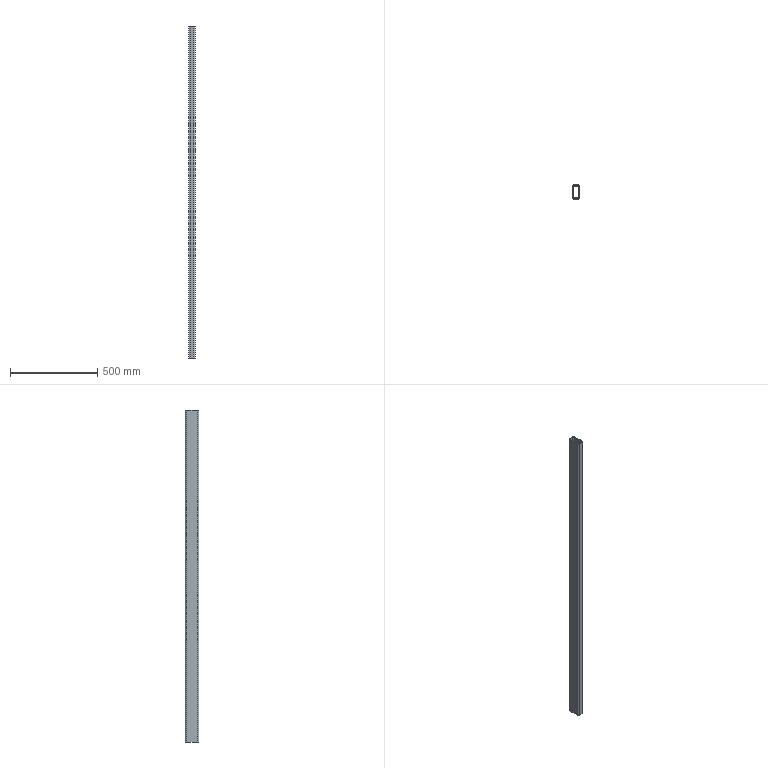Part | SolidWorks | features Extrusion 1 | 1 solid | 18 faces | box 40 x 80 x 1900 mm | volume 1967677 mm3 | plane 10 | cylinder 8 | commonest cylinder face diameters 10 x4 20 x4
STEP:
#1=CARTESIAN_POINT('',(-20.,-30.,1900.));
#2=VERTEX_POINT('',#1);
#3=CARTESIAN_POINT('',(-10.,-40.,1900.));
#4=VERTEX_POINT('',#3);
#5=CARTESIAN_POINT('',(-10.,-30.,1900.));
#6=DIRECTION('',(0.,0.,1.));
#7=DIRECTION('',(1.,0.,0.));
#8=AXIS2_PLACEMENT_3D('',#5,#6,#7);
#9=CIRCLE('',#8,10.);
#10=EDGE_CURVE('',#2,#4,#9,.T.);
#11=ORIENTED_EDGE('',*,*,#10,.T.);
#12=CARTESIAN_POINT('',(10.,-40.,1900.));
#13=VERTEX_POINT('',#12);
#14=CARTESIAN_POINT('',(-10.,-40.,1900.));
#15=DIRECTION('',(1.,0.,0.));
#16=VECTOR('',#15,1000.);
#17=LINE('',#14,#16);
#18=EDGE_CURVE('',#4,#13,#17,.T.);
#19=ORIENTED_EDGE('',*,*,#18,.T.);
#20=CARTESIAN_POINT('',(20.,-30.,1900.));
#21=VERTEX_POINT('',#20);
#22=CARTESIAN_POINT('',(10.,-30.,1900.));
#23=DIRECTION('',(0.,0.,1.));
#24=DIRECTION('',(1.,0.,0.));
#25=AXIS2_PLACEMENT_3D('',#22,#23,#24);
#26=CIRCLE('',#25,10.);
#27=EDGE_CURVE('',#13,#21,#26,.T.);
#28=ORIENTED_EDGE('',*,*,#27,.T.);
#29=CARTESIAN_POINT('',(20.,30.,1900.));
#30=VERTEX_POINT('',#29);
#31=CARTESIAN_POINT('',(20.,30.,1900.));
#32=DIRECTION('',(0.,-1.,0.));
#33=VECTOR('',#32,1000.);
#34=LINE('',#31,#33);
#35=EDGE_CURVE('',#30,#21,#34,.T.);
#36=ORIENTED_EDGE('',*,*,#35,.F.);
#37=CARTESIAN_POINT('',(10.,40.,1900.));
#38=VERTEX_POINT('',#37);
#39=CARTESIAN_POINT('',(10.,30.,1900.));
#40=DIRECTION('',(0.,0.,1.));
#41=DIRECTION('',(1.,0.,0.));
#42=AXIS2_PLACEMENT_3D('',#39,#40,#41);
#43=CIRCLE('',#42,10.);
#44=EDGE_CURVE('',#30,#38,#43,.T.);
#45=ORIENTED_EDGE('',*,*,#44,.T.);
#46=CARTESIAN_POINT('',(-10.,40.,1900.));
#47=VERTEX_POINT('',#46);
#48=CARTESIAN_POINT('',(10.,40.,1900.));
#49=DIRECTION('',(-1.,0.,0.));
#50=VECTOR('',#49,1000.);
#51=LINE('',#48,#50);
#52=EDGE_CURVE('',#38,#47,#51,.T.);
#53=ORIENTED_EDGE('',*,*,#52,.T.);
#54=CARTESIAN_POINT('',(-20.,30.,1900.));
#55=VERTEX_POINT('',#54);
#56=CARTESIAN_POINT('',(-10.,30.,1900.));
#57=DIRECTION('',(0.,0.,1.));
#58=DIRECTION('',(1.,0.,0.));
#59=AXIS2_PLACEMENT_3D('',#56,#57,#58);
#60=CIRCLE('',#59,10.);
#61=EDGE_CURVE('',#47,#55,#60,.T.);
#62=ORIENTED_EDGE('',*,*,#61,.T.);
#63=CARTESIAN_POINT('',(-20.,-30.,1900.));
#64=DIRECTION('',(0.,1.,0.));
#65=VECTOR('',#64,1000.);
#66=LINE('',#63,#65);
#67=EDGE_CURVE('',#2,#55,#66,.T.);
#68=ORIENTED_EDGE('',*,*,#67,.F.);
#69=EDGE_LOOP('',(#11,#19,#28,#36,#45,#53,#62,#68));
#70=FACE_OUTER_BOUND('',#69,.T.);
#71=CARTESIAN_POINT('',(-10.,-35.,1900.));
#72=VERTEX_POINT('',#71);
#73=CARTESIAN_POINT('',(10.,-35.,1900.));
#74=VERTEX_POINT('',#73);
#75=CARTESIAN_POINT('',(-10.,-35.,1900.));
#76=DIRECTION('',(1.,0.,0.));
#77=VECTOR('',#76,1000.);
#78=LINE('',#75,#77);
#79=EDGE_CURVE('',#72,#74,#78,.T.);
#80=ORIENTED_EDGE('',*,*,#79,.F.);
#81=CARTESIAN_POINT('',(-15.,-30.,1900.));
#82=VERTEX_POINT('',#81);
#83=CARTESIAN_POINT('',(-10.,-30.,1900.));
#84=DIRECTION('',(0.,0.,1.));
#85=DIRECTION('',(1.,0.,0.));
#86=AXIS2_PLACEMENT_3D('',#83,#84,#85);
#87=CIRCLE('',#86,5.);
#88=EDGE_CURVE('',#82,#72,#87,.T.);
#89=ORIENTED_EDGE('',*,*,#88,.F.);
#90=CARTESIAN_POINT('',(-15.,30.,1900.));
#91=VERTEX_POINT('',#90);
#92=CARTESIAN_POINT('',(-15.,-30.,1900.));
#93=DIRECTION('',(0.,1.,0.));
#94=VECTOR('',#93,1000.);
#95=LINE('',#92,#94);
#96=EDGE_CURVE('',#82,#91,#95,.T.);
#97=ORIENTED_EDGE('',*,*,#96,.T.);
#98=CARTESIAN_POINT('',(-10.,35.,1900.));
#99=VERTEX_POINT('',#98);
#100=CARTESIAN_POINT('',(-10.,30.,1900.));
#101=DIRECTION('',(0.,0.,1.));
#102=DIRECTION('',(1.,0.,0.));
#103=AXIS2_PLACEMENT_3D('',#100,#101,#102);
#104=CIRCLE('',#103,5.);
#105=EDGE_CURVE('',#99,#91,#104,.T.);
#106=ORIENTED_EDGE('',*,*,#105,.F.);
#107=CARTESIAN_POINT('',(10.,35.,1900.));
#108=VERTEX_POINT('',#107);
#109=CARTESIAN_POINT('',(10.,35.,1900.));
#110=DIRECTION('',(-1.,0.,0.));
#111=VECTOR('',#110,1000.);
#112=LINE('',#109,#111);
#113=EDGE_CURVE('',#108,#99,#112,.T.);
#114=ORIENTED_EDGE('',*,*,#113,.F.);
#115=CARTESIAN_POINT('',(15.,30.,1900.));
#116=VERTEX_POINT('',#115);
#117=CARTESIAN_POINT('',(10.,30.,1900.));
#118=DIRECTION('',(0.,0.,1.));
#119=DIRECTION('',(1.,0.,0.));
#120=AXIS2_PLACEMENT_3D('',#117,#118,#119);
#121=CIRCLE('',#120,5.);
#122=EDGE_CURVE('',#116,#108,#121,.T.);
#123=ORIENTED_EDGE('',*,*,#122,.F.);
#124=CARTESIAN_POINT('',(15.,-30.,1900.));
#125=VERTEX_POINT('',#124);
#126=CARTESIAN_POINT('',(15.,30.,1900.));
#127=DIRECTION('',(0.,-1.,0.));
#128=VECTOR('',#127,1000.);
#129=LINE('',#126,#128);
#130=EDGE_CURVE('',#116,#125,#129,.T.);
#131=ORIENTED_EDGE('',*,*,#130,.T.);
#132=CARTESIAN_POINT('',(10.,-30.,1900.));
#133=DIRECTION('',(0.,0.,1.));
#134=DIRECTION('',(1.,0.,0.));
#135=AXIS2_PLACEMENT_3D('',#132,#133,#134);
#136=CIRCLE('',#135,5.);
#137=EDGE_CURVE('',#74,#125,#136,.T.);
#138=ORIENTED_EDGE('',*,*,#137,.F.);
#139=EDGE_LOOP('',(#80,#89,#97,#106,#114,#123,#131,#138));
#140=FACE_BOUND('',#139,.T.);
#141=CARTESIAN_POINT('',(-10.,-30.,1900.));
#142=DIRECTION('',(0.,0.,1.));
#143=DIRECTION('',(1.,0.,0.));
#144=AXIS2_PLACEMENT_3D('',#141,#142,#143);
#145=PLANE('',#144);
#146=ADVANCED_FACE('',(#70,#140),#145,.T.);
#147=CARTESIAN_POINT('',(-20.,-30.,0.));
#148=VERTEX_POINT('',#147);
#149=CARTESIAN_POINT('',(-10.,-40.,0.));
#150=VERTEX_POINT('',#149);
#151=CARTESIAN_POINT('',(-10.,-30.,0.));
#152=DIRECTION('',(0.,0.,1.));
#153=DIRECTION('',(1.,0.,0.));
#154=AXIS2_PLACEMENT_3D('',#151,#152,#153);
#155=CIRCLE('',#154,10.);
#156=EDGE_CURVE('',#148,#150,#155,.T.);
#157=ORIENTED_EDGE('',*,*,#156,.F.);
#158=CARTESIAN_POINT('',(-20.,30.,0.));
#159=VERTEX_POINT('',#158);
#160=CARTESIAN_POINT('',(-20.,-30.,0.));
#161=DIRECTION('',(0.,1.,0.));
#162=VECTOR('',#161,1000.);
#163=LINE('',#160,#162);
#164=EDGE_CURVE('',#148,#159,#163,.T.);
#165=ORIENTED_EDGE('',*,*,#164,.T.);
#166=CARTESIAN_POINT('',(-10.,40.,0.));
#167=VERTEX_POINT('',#166);
#168=CARTESIAN_POINT('',(-10.,30.,0.));
#169=DIRECTION('',(0.,0.,1.));
#170=DIRECTION('',(1.,0.,0.));
#171=AXIS2_PLACEMENT_3D('',#168,#169,#170);
#172=CIRCLE('',#171,10.);
#173=EDGE_CURVE('',#167,#159,#172,.T.);
#174=ORIENTED_EDGE('',*,*,#173,.F.);
#175=CARTESIAN_POINT('',(10.,40.,0.));
#176=VERTEX_POINT('',#175);
#177=CARTESIAN_POINT('',(10.,40.,0.));
#178=DIRECTION('',(-1.,0.,0.));
#179=VECTOR('',#178,1000.);
#180=LINE('',#177,#179);
#181=EDGE_CURVE('',#176,#167,#180,.T.);
#182=ORIENTED_EDGE('',*,*,#181,.F.);
#183=CARTESIAN_POINT('',(20.,30.,0.));
#184=VERTEX_POINT('',#183);
#185=CARTESIAN_POINT('',(10.,30.,0.));
#186=DIRECTION('',(0.,0.,1.));
#187=DIRECTION('',(1.,0.,0.));
#188=AXIS2_PLACEMENT_3D('',#185,#186,#187);
#189=CIRCLE('',#188,10.);
#190=EDGE_CURVE('',#184,#176,#189,.T.);
#191=ORIENTED_EDGE('',*,*,#190,.F.);
#192=CARTESIAN_POINT('',(20.,-30.,0.));
#193=VERTEX_POINT('',#192);
#194=CARTESIAN_POINT('',(20.,30.,0.));
#195=DIRECTION('',(0.,-1.,0.));
#196=VECTOR('',#195,1000.);
#197=LINE('',#194,#196);
#198=EDGE_CURVE('',#184,#193,#197,.T.);
#199=ORIENTED_EDGE('',*,*,#198,.T.);
#200=CARTESIAN_POINT('',(10.,-40.,0.));
#201=VERTEX_POINT('',#200);
#202=CARTESIAN_POINT('',(10.,-30.,0.));
#203=DIRECTION('',(0.,0.,1.));
#204=DIRECTION('',(1.,0.,0.));
#205=AXIS2_PLACEMENT_3D('',#202,#203,#204);
#206=CIRCLE('',#205,10.);
#207=EDGE_CURVE('',#201,#193,#206,.T.);
#208=ORIENTED_EDGE('',*,*,#207,.F.);
#209=CARTESIAN_POINT('',(-10.,-40.,0.));
#210=DIRECTION('',(1.,0.,0.));
#211=VECTOR('',#210,1000.);
#212=LINE('',#209,#211);
#213=EDGE_CURVE('',#150,#201,#212,.T.);
#214=ORIENTED_EDGE('',*,*,#213,.F.);
#215=EDGE_LOOP('',(#157,#165,#174,#182,#191,#199,#208,#214));
#216=FACE_OUTER_BOUND('',#215,.T.);
#217=CARTESIAN_POINT('',(-15.,-30.,0.));
#218=VERTEX_POINT('',#217);
#219=CARTESIAN_POINT('',(-10.,-35.,0.));
#220=VERTEX_POINT('',#219);
#221=CARTESIAN_POINT('',(-10.,-30.,0.));
#222=DIRECTION('',(0.,0.,1.));
#223=DIRECTION('',(1.,0.,0.));
#224=AXIS2_PLACEMENT_3D('',#221,#222,#223);
#225=CIRCLE('',#224,5.);
#226=EDGE_CURVE('',#218,#220,#225,.T.);
#227=ORIENTED_EDGE('',*,*,#226,.T.);
#228=CARTESIAN_POINT('',(10.,-35.,0.));
#229=VERTEX_POINT('',#228);
#230=CARTESIAN_POINT('',(-10.,-35.,0.));
#231=DIRECTION('',(1.,0.,0.));
#232=VECTOR('',#231,1000.);
#233=LINE('',#230,#232);
#234=EDGE_CURVE('',#220,#229,#233,.T.);
#235=ORIENTED_EDGE('',*,*,#234,.T.);
#236=CARTESIAN_POINT('',(15.,-30.,0.));
#237=VERTEX_POINT('',#236);
#238=CARTESIAN_POINT('',(10.,-30.,0.));
#239=DIRECTION('',(0.,0.,1.));
#240=DIRECTION('',(1.,0.,0.));
#241=AXIS2_PLACEMENT_3D('',#238,#239,#240);
#242=CIRCLE('',#241,5.);
#243=EDGE_CURVE('',#229,#237,#242,.T.);
#244=ORIENTED_EDGE('',*,*,#243,.T.);
#245=CARTESIAN_POINT('',(15.,30.,0.));
#246=VERTEX_POINT('',#245);
#247=CARTESIAN_POINT('',(15.,30.,0.));
#248=DIRECTION('',(0.,-1.,0.));
#249=VECTOR('',#248,1000.);
#250=LINE('',#247,#249);
#251=EDGE_CURVE('',#246,#237,#250,.T.);
#252=ORIENTED_EDGE('',*,*,#251,.F.);
#253=CARTESIAN_POINT('',(10.,35.,0.));
#254=VERTEX_POINT('',#253);
#255=CARTESIAN_POINT('',(10.,30.,0.));
#256=DIRECTION('',(0.,0.,1.));
#257=DIRECTION('',(1.,0.,0.));
#258=AXIS2_PLACEMENT_3D('',#255,#256,#257);
#259=CIRCLE('',#258,5.);
#260=EDGE_CURVE('',#246,#254,#259,.T.);
#261=ORIENTED_EDGE('',*,*,#260,.T.);
#262=CARTESIAN_POINT('',(-10.,35.,0.));
#263=VERTEX_POINT('',#262);
#264=CARTESIAN_POINT('',(10.,35.,0.));
#265=DIRECTION('',(-1.,0.,0.));
#266=VECTOR('',#265,1000.);
#267=LINE('',#264,#266);
#268=EDGE_CURVE('',#254,#263,#267,.T.);
#269=ORIENTED_EDGE('',*,*,#268,.T.);
#270=CARTESIAN_POINT('',(-15.,30.,0.));
#271=VERTEX_POINT('',#270);
#272=CARTESIAN_POINT('',(-10.,30.,0.));
#273=DIRECTION('',(0.,0.,1.));
#274=DIRECTION('',(1.,0.,0.));
#275=AXIS2_PLACEMENT_3D('',#272,#273,#274);
#276=CIRCLE('',#275,5.);
#277=EDGE_CURVE('',#263,#271,#276,.T.);
#278=ORIENTED_EDGE('',*,*,#277,.T.);
#279=CARTESIAN_POINT('',(-15.,-30.,0.));
#280=DIRECTION('',(0.,1.,0.));
#281=VECTOR('',#280,1000.);
#282=LINE('',#279,#281);
#283=EDGE_CURVE('',#218,#271,#282,.T.);
#284=ORIENTED_EDGE('',*,*,#283,.F.);
#285=EDGE_LOOP('',(#227,#235,#244,#252,#261,#269,#278,#284));
#286=FACE_BOUND('',#285,.T.);
#287=CARTESIAN_POINT('',(-10.,-30.,0.));
#288=DIRECTION('',(0.,0.,1.));
#289=DIRECTION('',(1.,0.,0.));
#290=AXIS2_PLACEMENT_3D('',#287,#288,#289);
#291=PLANE('',#290);
#292=ADVANCED_FACE('',(#216,#286),#291,.F.);
#293=ORIENTED_EDGE('',*,*,#156,.T.);
#294=CARTESIAN_POINT('',(-10.,-40.,1900.));
#295=DIRECTION('',(0.,0.,-1.));
#296=VECTOR('',#295,1000.);
#297=LINE('',#294,#296);
#298=EDGE_CURVE('',#4,#150,#297,.T.);
#299=ORIENTED_EDGE('',*,*,#298,.F.);
#300=ORIENTED_EDGE('',*,*,#10,.F.);
#301=CARTESIAN_POINT('',(-20.,-30.,1900.));
#302=DIRECTION('',(0.,0.,-1.));
#303=VECTOR('',#302,1000.);
#304=LINE('',#301,#303);
#305=EDGE_CURVE('',#2,#148,#304,.T.);
#306=ORIENTED_EDGE('',*,*,#305,.T.);
#307=EDGE_LOOP('',(#293,#299,#300,#306));
#308=FACE_OUTER_BOUND('',#307,.T.);
#309=CARTESIAN_POINT('',(-10.,-30.,1900.));
#310=DIRECTION('',(0.,0.,-1.));
#311=DIRECTION('',(-1.,0.,0.));
#312=AXIS2_PLACEMENT_3D('',#309,#310,#311);
#313=CYLINDRICAL_SURFACE('',#312,10.);
#314=ADVANCED_FACE('',(#308),#313,.T.);
#315=ORIENTED_EDGE('',*,*,#213,.T.);
#316=CARTESIAN_POINT('',(10.,-40.,1900.));
#317=DIRECTION('',(0.,0.,-1.));
#318=VECTOR('',#317,1000.);
#319=LINE('',#316,#318);
#320=EDGE_CURVE('',#13,#201,#319,.T.);
#321=ORIENTED_EDGE('',*,*,#320,.F.);
#322=ORIENTED_EDGE('',*,*,#18,.F.);
#323=ORIENTED_EDGE('',*,*,#298,.T.);
#324=EDGE_LOOP('',(#315,#321,#322,#323));
#325=FACE_OUTER_BOUND('',#324,.T.);
#326=CARTESIAN_POINT('',(-10.,-40.,1900.));
#327=DIRECTION('',(0.,1.,0.));
#328=DIRECTION('',(0.,0.,1.));
#329=AXIS2_PLACEMENT_3D('',#326,#327,#328);
#330=PLANE('',#329);
#331=ADVANCED_FACE('',(#325),#330,.F.);
#332=ORIENTED_EDGE('',*,*,#207,.T.);
#333=CARTESIAN_POINT('',(20.,-30.,1900.));
#334=DIRECTION('',(0.,0.,-1.));
#335=VECTOR('',#334,1000.);
#336=LINE('',#333,#335);
#337=EDGE_CURVE('',#21,#193,#336,.T.);
#338=ORIENTED_EDGE('',*,*,#337,.F.);
#339=ORIENTED_EDGE('',*,*,#27,.F.);
#340=ORIENTED_EDGE('',*,*,#320,.T.);
#341=EDGE_LOOP('',(#332,#338,#339,#340));
#342=FACE_OUTER_BOUND('',#341,.T.);
#343=CARTESIAN_POINT('',(10.,-30.,1900.));
#344=DIRECTION('',(0.,0.,-1.));
#345=DIRECTION('',(-1.,0.,0.));
#346=AXIS2_PLACEMENT_3D('',#343,#344,#345);
#347=CYLINDRICAL_SURFACE('',#346,10.);
#348=ADVANCED_FACE('',(#342),#347,.T.);
#349=ORIENTED_EDGE('',*,*,#198,.F.);
#350=CARTESIAN_POINT('',(20.,30.,1900.));
#351=DIRECTION('',(0.,0.,-1.));
#352=VECTOR('',#351,1000.);
#353=LINE('',#350,#352);
#354=EDGE_CURVE('',#30,#184,#353,.T.);
#355=ORIENTED_EDGE('',*,*,#354,.F.);
#356=ORIENTED_EDGE('',*,*,#35,.T.);
#357=ORIENTED_EDGE('',*,*,#337,.T.);
#358=EDGE_LOOP('',(#349,#355,#356,#357));
#359=FACE_OUTER_BOUND('',#358,.T.);
#360=CARTESIAN_POINT('',(20.,30.,1900.));
#361=DIRECTION('',(1.,0.,0.));
#362=DIRECTION('',(0.,0.,-1.));
#363=AXIS2_PLACEMENT_3D('',#360,#361,#362);
#364=PLANE('',#363);
#365=ADVANCED_FACE('',(#359),#364,.T.);
#366=ORIENTED_EDGE('',*,*,#190,.T.);
#367=CARTESIAN_POINT('',(10.,40.,1900.));
#368=DIRECTION('',(0.,0.,-1.));
#369=VECTOR('',#368,1000.);
#370=LINE('',#367,#369);
#371=EDGE_CURVE('',#38,#176,#370,.T.);
#372=ORIENTED_EDGE('',*,*,#371,.F.);
#373=ORIENTED_EDGE('',*,*,#44,.F.);
#374=ORIENTED_EDGE('',*,*,#354,.T.);
#375=EDGE_LOOP('',(#366,#372,#373,#374));
#376=FACE_OUTER_BOUND('',#375,.T.);
#377=CARTESIAN_POINT('',(10.,30.,1900.));
#378=DIRECTION('',(0.,0.,-1.));
#379=DIRECTION('',(-1.,0.,0.));
#380=AXIS2_PLACEMENT_3D('',#377,#378,#379);
#381=CYLINDRICAL_SURFACE('',#380,10.);
#382=ADVANCED_FACE('',(#376),#381,.T.);
#383=ORIENTED_EDGE('',*,*,#181,.T.);
#384=CARTESIAN_POINT('',(-10.,40.,1900.));
#385=DIRECTION('',(0.,0.,-1.));
#386=VECTOR('',#385,1000.);
#387=LINE('',#384,#386);
#388=EDGE_CURVE('',#47,#167,#387,.T.);
#389=ORIENTED_EDGE('',*,*,#388,.F.);
#390=ORIENTED_EDGE('',*,*,#52,.F.);
#391=ORIENTED_EDGE('',*,*,#371,.T.);
#392=EDGE_LOOP('',(#383,#389,#390,#391));
#393=FACE_OUTER_BOUND('',#392,.T.);
#394=CARTESIAN_POINT('',(10.,40.,1900.));
#395=DIRECTION('',(0.,-1.,0.));
#396=DIRECTION('',(0.,0.,-1.));
#397=AXIS2_PLACEMENT_3D('',#394,#395,#396);
#398=PLANE('',#397);
#399=ADVANCED_FACE('',(#393),#398,.F.);
#400=ORIENTED_EDGE('',*,*,#173,.T.);
#401=CARTESIAN_POINT('',(-20.,30.,1900.));
#402=DIRECTION('',(0.,0.,-1.));
#403=VECTOR('',#402,1000.);
#404=LINE('',#401,#403);
#405=EDGE_CURVE('',#55,#159,#404,.T.);
#406=ORIENTED_EDGE('',*,*,#405,.F.);
#407=ORIENTED_EDGE('',*,*,#61,.F.);
#408=ORIENTED_EDGE('',*,*,#388,.T.);
#409=EDGE_LOOP('',(#400,#406,#407,#408));
#410=FACE_OUTER_BOUND('',#409,.T.);
#411=CARTESIAN_POINT('',(-10.,30.,1900.));
#412=DIRECTION('',(0.,0.,-1.));
#413=DIRECTION('',(-1.,0.,0.));
#414=AXIS2_PLACEMENT_3D('',#411,#412,#413);
#415=CYLINDRICAL_SURFACE('',#414,10.);
#416=ADVANCED_FACE('',(#410),#415,.T.);
#417=ORIENTED_EDGE('',*,*,#164,.F.);
#418=ORIENTED_EDGE('',*,*,#305,.F.);
#419=ORIENTED_EDGE('',*,*,#67,.T.);
#420=ORIENTED_EDGE('',*,*,#405,.T.);
#421=EDGE_LOOP('',(#417,#418,#419,#420));
#422=FACE_OUTER_BOUND('',#421,.T.);
#423=CARTESIAN_POINT('',(-20.,-30.,1900.));
#424=DIRECTION('',(-1.,0.,0.));
#425=DIRECTION('',(0.,0.,1.));
#426=AXIS2_PLACEMENT_3D('',#423,#424,#425);
#427=PLANE('',#426);
#428=ADVANCED_FACE('',(#422),#427,.T.);
#429=ORIENTED_EDGE('',*,*,#226,.F.);
#430=CARTESIAN_POINT('',(-15.,-30.,1900.));
#431=DIRECTION('',(0.,0.,-1.));
#432=VECTOR('',#431,1000.);
#433=LINE('',#430,#432);
#434=EDGE_CURVE('',#82,#218,#433,.T.);
#435=ORIENTED_EDGE('',*,*,#434,.F.);
#436=ORIENTED_EDGE('',*,*,#88,.T.);
#437=CARTESIAN_POINT('',(-10.,-35.,1900.));
#438=DIRECTION('',(0.,0.,-1.));
#439=VECTOR('',#438,1000.);
#440=LINE('',#437,#439);
#441=EDGE_CURVE('',#72,#220,#440,.T.);
#442=ORIENTED_EDGE('',*,*,#441,.T.);
#443=EDGE_LOOP('',(#429,#435,#436,#442));
#444=FACE_OUTER_BOUND('',#443,.T.);
#445=CARTESIAN_POINT('',(-10.,-30.,1900.));
#446=DIRECTION('',(0.,0.,-1.));
#447=DIRECTION('',(-1.,0.,0.));
#448=AXIS2_PLACEMENT_3D('',#445,#446,#447);
#449=CYLINDRICAL_SURFACE('',#448,5.);
#450=ADVANCED_FACE('',(#444),#449,.F.);
#451=ORIENTED_EDGE('',*,*,#234,.F.);
#452=ORIENTED_EDGE('',*,*,#441,.F.);
#453=ORIENTED_EDGE('',*,*,#79,.T.);
#454=CARTESIAN_POINT('',(10.,-35.,1900.));
#455=DIRECTION('',(0.,0.,-1.));
#456=VECTOR('',#455,1000.);
#457=LINE('',#454,#456);
#458=EDGE_CURVE('',#74,#229,#457,.T.);
#459=ORIENTED_EDGE('',*,*,#458,.T.);
#460=EDGE_LOOP('',(#451,#452,#453,#459));
#461=FACE_OUTER_BOUND('',#460,.T.);
#462=CARTESIAN_POINT('',(-10.,-35.,1900.));
#463=DIRECTION('',(0.,1.,0.));
#464=DIRECTION('',(0.,0.,1.));
#465=AXIS2_PLACEMENT_3D('',#462,#463,#464);
#466=PLANE('',#465);
#467=ADVANCED_FACE('',(#461),#466,.T.);
#468=ORIENTED_EDGE('',*,*,#243,.F.);
#469=ORIENTED_EDGE('',*,*,#458,.F.);
#470=ORIENTED_EDGE('',*,*,#137,.T.);
#471=CARTESIAN_POINT('',(15.,-30.,1900.));
#472=DIRECTION('',(0.,0.,-1.));
#473=VECTOR('',#472,1000.);
#474=LINE('',#471,#473);
#475=EDGE_CURVE('',#125,#237,#474,.T.);
#476=ORIENTED_EDGE('',*,*,#475,.T.);
#477=EDGE_LOOP('',(#468,#469,#470,#476));
#478=FACE_OUTER_BOUND('',#477,.T.);
#479=CARTESIAN_POINT('',(10.,-30.,1900.));
#480=DIRECTION('',(0.,0.,-1.));
#481=DIRECTION('',(-1.,0.,0.));
#482=AXIS2_PLACEMENT_3D('',#479,#480,#481);
#483=CYLINDRICAL_SURFACE('',#482,5.);
#484=ADVANCED_FACE('',(#478),#483,.F.);
#485=ORIENTED_EDGE('',*,*,#251,.T.);
#486=ORIENTED_EDGE('',*,*,#475,.F.);
#487=ORIENTED_EDGE('',*,*,#130,.F.);
#488=CARTESIAN_POINT('',(15.,30.,1900.));
#489=DIRECTION('',(0.,0.,-1.));
#490=VECTOR('',#489,1000.);
#491=LINE('',#488,#490);
#492=EDGE_CURVE('',#116,#246,#491,.T.);
#493=ORIENTED_EDGE('',*,*,#492,.T.);
#494=EDGE_LOOP('',(#485,#486,#487,#493));
#495=FACE_OUTER_BOUND('',#494,.T.);
#496=CARTESIAN_POINT('',(15.,30.,1900.));
#497=DIRECTION('',(1.,0.,0.));
#498=DIRECTION('',(0.,0.,-1.));
#499=AXIS2_PLACEMENT_3D('',#496,#497,#498);
#500=PLANE('',#499);
#501=ADVANCED_FACE('',(#495),#500,.F.);
#502=ORIENTED_EDGE('',*,*,#260,.F.);
#503=ORIENTED_EDGE('',*,*,#492,.F.);
#504=ORIENTED_EDGE('',*,*,#122,.T.);
#505=CARTESIAN_POINT('',(10.,35.,1900.));
#506=DIRECTION('',(0.,0.,-1.));
#507=VECTOR('',#506,1000.);
#508=LINE('',#505,#507);
#509=EDGE_CURVE('',#108,#254,#508,.T.);
#510=ORIENTED_EDGE('',*,*,#509,.T.);
#511=EDGE_LOOP('',(#502,#503,#504,#510));
#512=FACE_OUTER_BOUND('',#511,.T.);
#513=CARTESIAN_POINT('',(10.,30.,1900.));
#514=DIRECTION('',(0.,0.,-1.));
#515=DIRECTION('',(-1.,0.,0.));
#516=AXIS2_PLACEMENT_3D('',#513,#514,#515);
#517=CYLINDRICAL_SURFACE('',#516,5.);
#518=ADVANCED_FACE('',(#512),#517,.F.);
#519=ORIENTED_EDGE('',*,*,#268,.F.);
#520=ORIENTED_EDGE('',*,*,#509,.F.);
#521=ORIENTED_EDGE('',*,*,#113,.T.);
#522=CARTESIAN_POINT('',(-10.,35.,1900.));
#523=DIRECTION('',(0.,0.,-1.));
#524=VECTOR('',#523,1000.);
#525=LINE('',#522,#524);
#526=EDGE_CURVE('',#99,#263,#525,.T.);
#527=ORIENTED_EDGE('',*,*,#526,.T.);
#528=EDGE_LOOP('',(#519,#520,#521,#527));
#529=FACE_OUTER_BOUND('',#528,.T.);
#530=CARTESIAN_POINT('',(10.,35.,1900.));
#531=DIRECTION('',(0.,-1.,0.));
#532=DIRECTION('',(0.,0.,-1.));
#533=AXIS2_PLACEMENT_3D('',#530,#531,#532);
#534=PLANE('',#533);
#535=ADVANCED_FACE('',(#529),#534,.T.);
#536=ORIENTED_EDGE('',*,*,#277,.F.);
#537=ORIENTED_EDGE('',*,*,#526,.F.);
#538=ORIENTED_EDGE('',*,*,#105,.T.);
#539=CARTESIAN_POINT('',(-15.,30.,1900.));
#540=DIRECTION('',(0.,0.,-1.));
#541=VECTOR('',#540,1000.);
#542=LINE('',#539,#541);
#543=EDGE_CURVE('',#91,#271,#542,.T.);
#544=ORIENTED_EDGE('',*,*,#543,.T.);
#545=EDGE_LOOP('',(#536,#537,#538,#544));
#546=FACE_OUTER_BOUND('',#545,.T.);
#547=CARTESIAN_POINT('',(-10.,30.,1900.));
#548=DIRECTION('',(0.,0.,-1.));
#549=DIRECTION('',(-1.,0.,0.));
#550=AXIS2_PLACEMENT_3D('',#547,#548,#549);
#551=CYLINDRICAL_SURFACE('',#550,5.);
#552=ADVANCED_FACE('',(#546),#551,.F.);
#553=ORIENTED_EDGE('',*,*,#283,.T.);
#554=ORIENTED_EDGE('',*,*,#543,.F.);
#555=ORIENTED_EDGE('',*,*,#96,.F.);
#556=ORIENTED_EDGE('',*,*,#434,.T.);
#557=EDGE_LOOP('',(#553,#554,#555,#556));
#558=FACE_OUTER_BOUND('',#557,.T.);
#559=CARTESIAN_POINT('',(-15.,-30.,1900.));
#560=DIRECTION('',(-1.,0.,0.));
#561=DIRECTION('',(0.,0.,1.));
#562=AXIS2_PLACEMENT_3D('',#559,#560,#561);
#563=PLANE('',#562);
#564=ADVANCED_FACE('',(#558),#563,.F.);
#565=CLOSED_SHELL('',(#146,#292,#314,#331,#348,#365,#382,#399,#416,#428,#450,#467,#484,#501,#518,#535,#552,#564));
#566=MANIFOLD_SOLID_BREP('',#565);
#567=CARTESIAN_POINT('',(0.,0.,0.));
#568=DIRECTION('',(0.,0.,1.));
#569=DIRECTION('',(1.,0.,0.));
#570=AXIS2_PLACEMENT_3D('',#567,#568,#569);
#571=(LENGTH_UNIT()NAMED_UNIT(*)SI_UNIT(.MILLI.,.METRE.));
#572=UNCERTAINTY_MEASURE_WITH_UNIT(LENGTH_MEASURE(0.00001),#571,'','');
#573=(NAMED_UNIT(*)PLANE_ANGLE_UNIT()SI_UNIT($,.RADIAN.));
#574=(NAMED_UNIT(*)SI_UNIT($,.STERADIAN.)SOLID_ANGLE_UNIT());
#575=(GEOMETRIC_REPRESENTATION_CONTEXT(3)GLOBAL_UNCERTAINTY_ASSIGNED_CONTEXT((#572))GLOBAL_UNIT_ASSIGNED_CONTEXT((#571,#573,#574))REPRESENTATION_CONTEXT('',''));
#576=ADVANCED_BREP_SHAPE_REPRESENTATION('',(#566,#570),#575);